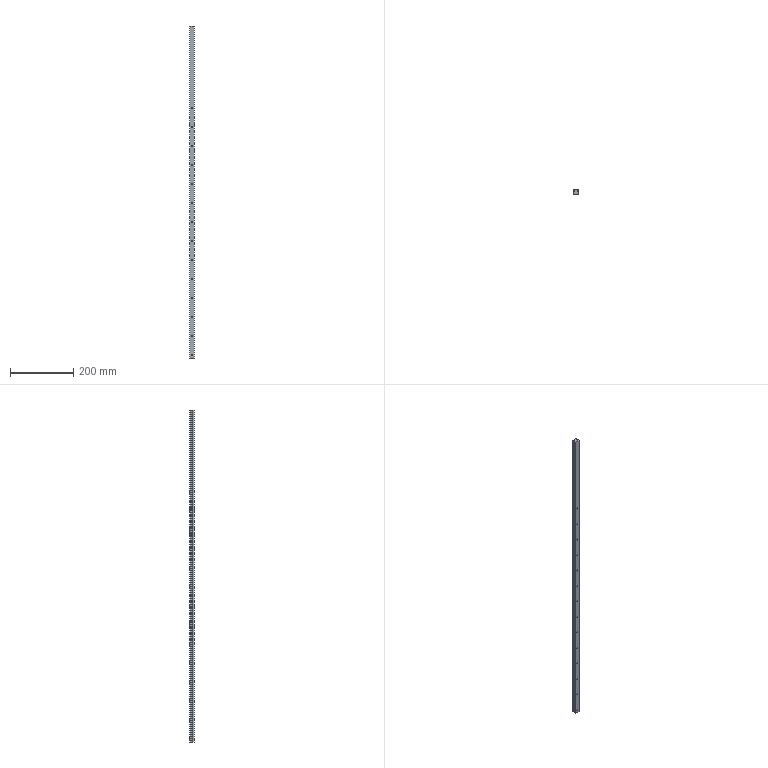Part | SolidWorks | features BaseBody 1 | 1 solid | 96 faces | box 15 x 15 x 1050 mm | volume 206865 mm3 | cylinder 62 | plane 34 | commonest cylinder face diameters 4.5 x28 7.5 x28 1.459 x6